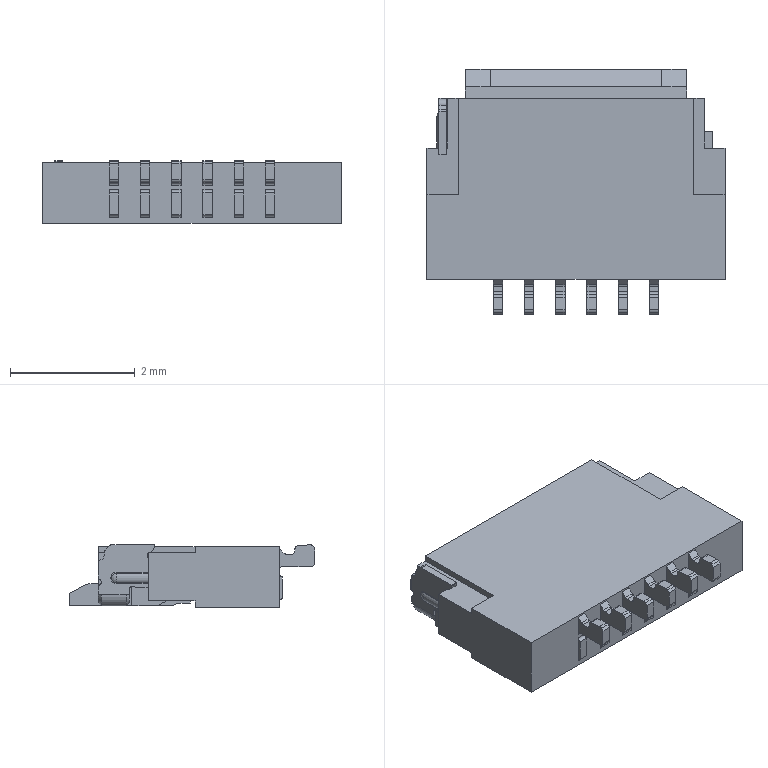Part | Creo | 1 solid | 342 faces | box 4.77 x 3.923 x 1 mm | volume 9.925 mm3 | plane 244 | cylinder 92 | sphere 2 | cone 2 | spline 1 | torus 1 | commonest cylinder face diameters 0.1 x70 0.2 x14 0.04 x2 0.28 x2 0.02 x1 0.125 x1